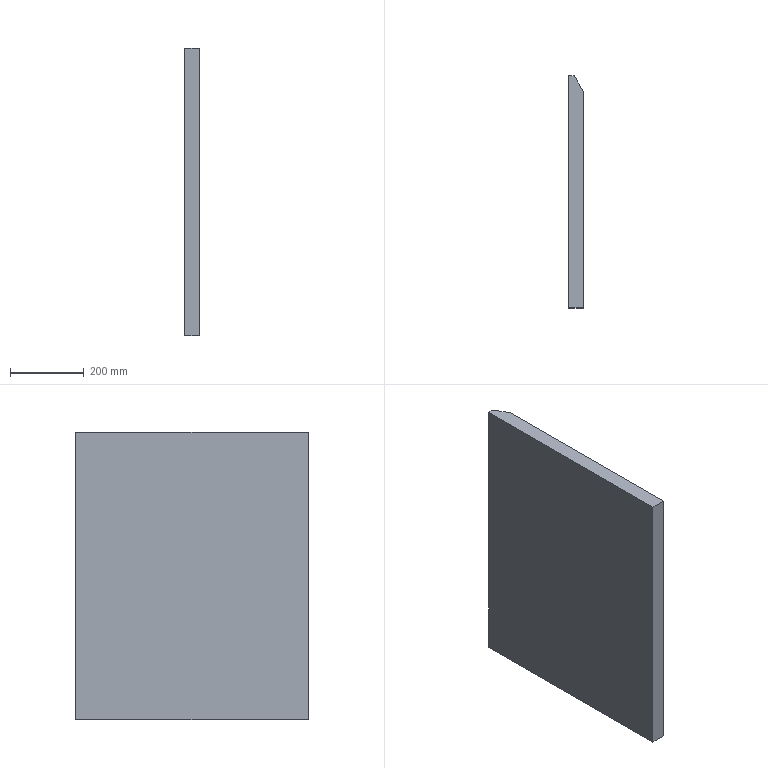Part | SolidWorks | features CutThin 1, Extrusion 1 | 1 solid | 17 faces | box 40 x 630 x 780 mm | volume 19233148 mm3 | plane 17
STEP:
#1=CARTESIAN_POINT('',(15.,0.,0.));
#2=VERTEX_POINT('',#1);
#3=CARTESIAN_POINT('',(0.,0.,0.));
#4=VERTEX_POINT('',#3);
#5=CARTESIAN_POINT('',(0.,0.,0.));
#6=DIRECTION('',(-1.,0.,0.));
#7=VECTOR('',#6,1000.);
#8=LINE('',#5,#7);
#9=EDGE_CURVE('',#2,#4,#8,.T.);
#10=ORIENTED_EDGE('',*,*,#9,.T.);
#11=CARTESIAN_POINT('',(0.,0.,780.));
#12=VERTEX_POINT('',#11);
#13=CARTESIAN_POINT('',(0.,0.,780.));
#14=DIRECTION('',(0.,0.,-1.));
#15=VECTOR('',#14,1000.);
#16=LINE('',#13,#15);
#17=EDGE_CURVE('',#12,#4,#16,.T.);
#18=ORIENTED_EDGE('',*,*,#17,.F.);
#19=CARTESIAN_POINT('',(15.,0.,780.));
#20=VERTEX_POINT('',#19);
#21=CARTESIAN_POINT('',(0.,0.,780.));
#22=DIRECTION('',(-1.,0.,0.));
#23=VECTOR('',#22,1000.);
#24=LINE('',#21,#23);
#25=EDGE_CURVE('',#20,#12,#24,.T.);
#26=ORIENTED_EDGE('',*,*,#25,.F.);
#27=CARTESIAN_POINT('',(15.,0.,780.));
#28=DIRECTION('',(0.,0.,-1.));
#29=VECTOR('',#28,1000.);
#30=LINE('',#27,#29);
#31=EDGE_CURVE('',#20,#2,#30,.T.);
#32=ORIENTED_EDGE('',*,*,#31,.T.);
#33=EDGE_LOOP('',(#10,#18,#26,#32));
#34=FACE_OUTER_BOUND('',#33,.T.);
#35=CARTESIAN_POINT('',(0.,0.,780.));
#36=DIRECTION('',(0.,-1.,0.));
#37=DIRECTION('',(0.,0.,-1.));
#38=AXIS2_PLACEMENT_3D('',#35,#36,#37);
#39=PLANE('',#38);
#40=ADVANCED_FACE('',(#34),#39,.F.);
#41=CARTESIAN_POINT('',(0.,-630.,0.));
#42=VERTEX_POINT('',#41);
#43=CARTESIAN_POINT('',(0.,0.,0.));
#44=DIRECTION('',(0.,-1.,0.));
#45=VECTOR('',#44,1000.);
#46=LINE('',#43,#45);
#47=EDGE_CURVE('',#4,#42,#46,.T.);
#48=ORIENTED_EDGE('',*,*,#47,.T.);
#49=CARTESIAN_POINT('',(0.,-630.,780.));
#50=VERTEX_POINT('',#49);
#51=CARTESIAN_POINT('',(0.,-630.,780.));
#52=DIRECTION('',(0.,0.,-1.));
#53=VECTOR('',#52,1000.);
#54=LINE('',#51,#53);
#55=EDGE_CURVE('',#50,#42,#54,.T.);
#56=ORIENTED_EDGE('',*,*,#55,.F.);
#57=CARTESIAN_POINT('',(0.,0.,780.));
#58=DIRECTION('',(0.,-1.,0.));
#59=VECTOR('',#58,1000.);
#60=LINE('',#57,#59);
#61=EDGE_CURVE('',#12,#50,#60,.T.);
#62=ORIENTED_EDGE('',*,*,#61,.F.);
#63=ORIENTED_EDGE('',*,*,#17,.T.);
#64=EDGE_LOOP('',(#48,#56,#62,#63));
#65=FACE_OUTER_BOUND('',#64,.T.);
#66=CARTESIAN_POINT('',(0.,0.,780.));
#67=DIRECTION('',(1.,0.,0.));
#68=DIRECTION('',(0.,1.,0.));
#69=AXIS2_PLACEMENT_3D('',#66,#67,#68);
#70=PLANE('',#69);
#71=ADVANCED_FACE('',(#65),#70,.F.);
#72=CARTESIAN_POINT('',(40.,-630.,0.));
#73=VERTEX_POINT('',#72);
#74=CARTESIAN_POINT('',(0.,-630.,0.));
#75=DIRECTION('',(1.,0.,0.));
#76=VECTOR('',#75,1000.);
#77=LINE('',#74,#76);
#78=EDGE_CURVE('',#42,#73,#77,.T.);
#79=ORIENTED_EDGE('',*,*,#78,.T.);
#80=CARTESIAN_POINT('',(40.,-630.,780.));
#81=VERTEX_POINT('',#80);
#82=CARTESIAN_POINT('',(40.,-630.,780.));
#83=DIRECTION('',(0.,0.,-1.));
#84=VECTOR('',#83,1000.);
#85=LINE('',#82,#84);
#86=EDGE_CURVE('',#81,#73,#85,.T.);
#87=ORIENTED_EDGE('',*,*,#86,.F.);
#88=CARTESIAN_POINT('',(0.,-630.,780.));
#89=DIRECTION('',(1.,0.,0.));
#90=VECTOR('',#89,1000.);
#91=LINE('',#88,#90);
#92=EDGE_CURVE('',#50,#81,#91,.T.);
#93=ORIENTED_EDGE('',*,*,#92,.F.);
#94=ORIENTED_EDGE('',*,*,#55,.T.);
#95=EDGE_LOOP('',(#79,#87,#93,#94));
#96=FACE_OUTER_BOUND('',#95,.T.);
#97=CARTESIAN_POINT('',(0.,-630.,780.));
#98=DIRECTION('',(0.,1.,0.));
#99=DIRECTION('',(0.,0.,1.));
#100=AXIS2_PLACEMENT_3D('',#97,#98,#99);
#101=PLANE('',#100);
#102=ADVANCED_FACE('',(#96),#101,.F.);
#103=CARTESIAN_POINT('',(40.,-144.501,439.2));
#104=VERTEX_POINT('',#103);
#105=CARTESIAN_POINT('',(40.,-144.501,340.8));
#106=VERTEX_POINT('',#105);
#107=CARTESIAN_POINT('',(40.,-144.501,438.));
#108=DIRECTION('',(0.,0.,-1.));
#109=VECTOR('',#108,1000.);
#110=LINE('',#107,#109);
#111=EDGE_CURVE('',#104,#106,#110,.T.);
#112=ORIENTED_EDGE('',*,*,#111,.F.);
#113=CARTESIAN_POINT('',(40.,-102.101,439.2));
#114=VERTEX_POINT('',#113);
#115=CARTESIAN_POINT('',(40.,-103.301,439.2));
#116=DIRECTION('',(0.,-1.,0.));
#117=VECTOR('',#116,1000.);
#118=LINE('',#115,#117);
#119=EDGE_CURVE('',#114,#104,#118,.T.);
#120=ORIENTED_EDGE('',*,*,#119,.F.);
#121=CARTESIAN_POINT('',(40.,-102.101,340.8));
#122=VERTEX_POINT('',#121);
#123=CARTESIAN_POINT('',(40.,-102.101,438.));
#124=DIRECTION('',(0.,0.,1.));
#125=VECTOR('',#124,1000.);
#126=LINE('',#123,#125);
#127=EDGE_CURVE('',#122,#114,#126,.T.);
#128=ORIENTED_EDGE('',*,*,#127,.F.);
#129=CARTESIAN_POINT('',(40.,-103.301,340.8));
#130=DIRECTION('',(0.,1.,0.));
#131=VECTOR('',#130,1000.);
#132=LINE('',#129,#131);
#133=EDGE_CURVE('',#106,#122,#132,.T.);
#134=ORIENTED_EDGE('',*,*,#133,.F.);
#135=EDGE_LOOP('',(#112,#120,#128,#134));
#136=FACE_BOUND('',#135,.T.);
#137=CARTESIAN_POINT('',(40.,-43.301,0.));
#138=VERTEX_POINT('',#137);
#139=CARTESIAN_POINT('',(40.,-630.,0.));
#140=DIRECTION('',(0.,1.,0.));
#141=VECTOR('',#140,1000.);
#142=LINE('',#139,#141);
#143=EDGE_CURVE('',#73,#138,#142,.T.);
#144=ORIENTED_EDGE('',*,*,#143,.T.);
#145=CARTESIAN_POINT('',(40.,-43.301,780.));
#146=VERTEX_POINT('',#145);
#147=CARTESIAN_POINT('',(40.,-43.301,780.));
#148=DIRECTION('',(0.,0.,-1.));
#149=VECTOR('',#148,1000.);
#150=LINE('',#147,#149);
#151=EDGE_CURVE('',#146,#138,#150,.T.);
#152=ORIENTED_EDGE('',*,*,#151,.F.);
#153=CARTESIAN_POINT('',(40.,-630.,780.));
#154=DIRECTION('',(0.,1.,0.));
#155=VECTOR('',#154,1000.);
#156=LINE('',#153,#155);
#157=EDGE_CURVE('',#81,#146,#156,.T.);
#158=ORIENTED_EDGE('',*,*,#157,.F.);
#159=ORIENTED_EDGE('',*,*,#86,.T.);
#160=EDGE_LOOP('',(#144,#152,#158,#159));
#161=FACE_OUTER_BOUND('',#160,.T.);
#162=CARTESIAN_POINT('',(40.,-630.,780.));
#163=DIRECTION('',(-1.,0.,0.));
#164=DIRECTION('',(0.,-1.,0.));
#165=AXIS2_PLACEMENT_3D('',#162,#163,#164);
#166=PLANE('',#165);
#167=ADVANCED_FACE('',(#136,#161),#166,.F.);
#168=CARTESIAN_POINT('',(15.,0.,0.));
#169=DIRECTION('',(-0.5,0.866,0.));
#170=VECTOR('',#169,1000.);
#171=LINE('',#168,#170);
#172=EDGE_CURVE('',#138,#2,#171,.T.);
#173=ORIENTED_EDGE('',*,*,#172,.T.);
#174=ORIENTED_EDGE('',*,*,#31,.F.);
#175=CARTESIAN_POINT('',(15.,0.,780.));
#176=DIRECTION('',(-0.5,0.866,0.));
#177=VECTOR('',#176,1000.);
#178=LINE('',#175,#177);
#179=EDGE_CURVE('',#146,#20,#178,.T.);
#180=ORIENTED_EDGE('',*,*,#179,.F.);
#181=ORIENTED_EDGE('',*,*,#151,.T.);
#182=EDGE_LOOP('',(#173,#174,#180,#181));
#183=FACE_OUTER_BOUND('',#182,.T.);
#184=CARTESIAN_POINT('',(15.,0.,780.));
#185=DIRECTION('',(-0.866,-0.5,0.));
#186=DIRECTION('',(0.5,-0.866,0.));
#187=AXIS2_PLACEMENT_3D('',#184,#185,#186);
#188=PLANE('',#187);
#189=ADVANCED_FACE('',(#183),#188,.F.);
#190=ORIENTED_EDGE('',*,*,#25,.T.);
#191=ORIENTED_EDGE('',*,*,#61,.T.);
#192=ORIENTED_EDGE('',*,*,#92,.T.);
#193=ORIENTED_EDGE('',*,*,#157,.T.);
#194=ORIENTED_EDGE('',*,*,#179,.T.);
#195=EDGE_LOOP('',(#190,#191,#192,#193,#194));
#196=FACE_OUTER_BOUND('',#195,.T.);
#197=CARTESIAN_POINT('',(0.,0.,780.));
#198=DIRECTION('',(0.,0.,1.));
#199=DIRECTION('',(1.,0.,0.));
#200=AXIS2_PLACEMENT_3D('',#197,#198,#199);
#201=PLANE('',#200);
#202=ADVANCED_FACE('',(#196),#201,.T.);
#203=ORIENTED_EDGE('',*,*,#9,.F.);
#204=ORIENTED_EDGE('',*,*,#172,.F.);
#205=ORIENTED_EDGE('',*,*,#143,.F.);
#206=ORIENTED_EDGE('',*,*,#78,.F.);
#207=ORIENTED_EDGE('',*,*,#47,.F.);
#208=EDGE_LOOP('',(#203,#204,#205,#206,#207));
#209=FACE_OUTER_BOUND('',#208,.T.);
#210=CARTESIAN_POINT('',(0.,0.,0.));
#211=DIRECTION('',(0.,0.,1.));
#212=DIRECTION('',(1.,0.,0.));
#213=AXIS2_PLACEMENT_3D('',#210,#211,#212);
#214=PLANE('',#213);
#215=ADVANCED_FACE('',(#209),#214,.F.);
#216=ORIENTED_EDGE('',*,*,#119,.T.);
#217=CARTESIAN_POINT('',(38.,-144.501,439.2));
#218=VERTEX_POINT('',#217);
#219=CARTESIAN_POINT('',(38.,-144.501,439.2));
#220=DIRECTION('',(1.,0.,0.));
#221=VECTOR('',#220,1000.);
#222=LINE('',#219,#221);
#223=EDGE_CURVE('',#218,#104,#222,.T.);
#224=ORIENTED_EDGE('',*,*,#223,.F.);
#225=CARTESIAN_POINT('',(38.,-102.101,439.2));
#226=VERTEX_POINT('',#225);
#227=CARTESIAN_POINT('',(38.,-103.301,439.2));
#228=DIRECTION('',(0.,-1.,0.));
#229=VECTOR('',#228,1000.);
#230=LINE('',#227,#229);
#231=EDGE_CURVE('',#226,#218,#230,.T.);
#232=ORIENTED_EDGE('',*,*,#231,.F.);
#233=CARTESIAN_POINT('',(38.,-102.101,439.2));
#234=DIRECTION('',(1.,0.,0.));
#235=VECTOR('',#234,1000.);
#236=LINE('',#233,#235);
#237=EDGE_CURVE('',#226,#114,#236,.T.);
#238=ORIENTED_EDGE('',*,*,#237,.T.);
#239=EDGE_LOOP('',(#216,#224,#232,#238));
#240=FACE_OUTER_BOUND('',#239,.T.);
#241=CARTESIAN_POINT('',(38.,-103.301,439.2));
#242=DIRECTION('',(0.,0.,1.));
#243=DIRECTION('',(1.,0.,0.));
#244=AXIS2_PLACEMENT_3D('',#241,#242,#243);
#245=PLANE('',#244);
#246=ADVANCED_FACE('',(#240),#245,.F.);
#247=ORIENTED_EDGE('',*,*,#127,.T.);
#248=ORIENTED_EDGE('',*,*,#237,.F.);
#249=CARTESIAN_POINT('',(38.,-102.101,340.8));
#250=VERTEX_POINT('',#249);
#251=CARTESIAN_POINT('',(38.,-102.101,438.));
#252=DIRECTION('',(0.,0.,1.));
#253=VECTOR('',#252,1000.);
#254=LINE('',#251,#253);
#255=EDGE_CURVE('',#250,#226,#254,.T.);
#256=ORIENTED_EDGE('',*,*,#255,.F.);
#257=CARTESIAN_POINT('',(38.,-102.101,340.8));
#258=DIRECTION('',(1.,0.,0.));
#259=VECTOR('',#258,1000.);
#260=LINE('',#257,#259);
#261=EDGE_CURVE('',#250,#122,#260,.T.);
#262=ORIENTED_EDGE('',*,*,#261,.T.);
#263=EDGE_LOOP('',(#247,#248,#256,#262));
#264=FACE_OUTER_BOUND('',#263,.T.);
#265=CARTESIAN_POINT('',(38.,-102.101,438.));
#266=DIRECTION('',(0.,1.,0.));
#267=DIRECTION('',(0.,0.,1.));
#268=AXIS2_PLACEMENT_3D('',#265,#266,#267);
#269=PLANE('',#268);
#270=ADVANCED_FACE('',(#264),#269,.F.);
#271=ORIENTED_EDGE('',*,*,#133,.T.);
#272=ORIENTED_EDGE('',*,*,#261,.F.);
#273=CARTESIAN_POINT('',(38.,-144.501,340.8));
#274=VERTEX_POINT('',#273);
#275=CARTESIAN_POINT('',(38.,-103.301,340.8));
#276=DIRECTION('',(0.,1.,0.));
#277=VECTOR('',#276,1000.);
#278=LINE('',#275,#277);
#279=EDGE_CURVE('',#274,#250,#278,.T.);
#280=ORIENTED_EDGE('',*,*,#279,.F.);
#281=CARTESIAN_POINT('',(38.,-144.501,340.8));
#282=DIRECTION('',(1.,0.,0.));
#283=VECTOR('',#282,1000.);
#284=LINE('',#281,#283);
#285=EDGE_CURVE('',#274,#106,#284,.T.);
#286=ORIENTED_EDGE('',*,*,#285,.T.);
#287=EDGE_LOOP('',(#271,#272,#280,#286));
#288=FACE_OUTER_BOUND('',#287,.T.);
#289=CARTESIAN_POINT('',(38.,-103.301,340.8));
#290=DIRECTION('',(0.,0.,-1.));
#291=DIRECTION('',(0.,1.,0.));
#292=AXIS2_PLACEMENT_3D('',#289,#290,#291);
#293=PLANE('',#292);
#294=ADVANCED_FACE('',(#288),#293,.F.);
#295=ORIENTED_EDGE('',*,*,#111,.T.);
#296=ORIENTED_EDGE('',*,*,#285,.F.);
#297=CARTESIAN_POINT('',(38.,-144.501,438.));
#298=DIRECTION('',(0.,0.,-1.));
#299=VECTOR('',#298,1000.);
#300=LINE('',#297,#299);
#301=EDGE_CURVE('',#218,#274,#300,.T.);
#302=ORIENTED_EDGE('',*,*,#301,.F.);
#303=ORIENTED_EDGE('',*,*,#223,.T.);
#304=EDGE_LOOP('',(#295,#296,#302,#303));
#305=FACE_OUTER_BOUND('',#304,.T.);
#306=CARTESIAN_POINT('',(38.,-144.501,438.));
#307=DIRECTION('',(0.,-1.,0.));
#308=DIRECTION('',(1.,0.,0.));
#309=AXIS2_PLACEMENT_3D('',#306,#307,#308);
#310=PLANE('',#309);
#311=ADVANCED_FACE('',(#305),#310,.F.);
#312=CARTESIAN_POINT('',(38.,-103.301,342.));
#313=VERTEX_POINT('',#312);
#314=CARTESIAN_POINT('',(38.,-103.301,438.));
#315=VERTEX_POINT('',#314);
#316=CARTESIAN_POINT('',(38.,-103.301,438.));
#317=DIRECTION('',(0.,0.,1.));
#318=VECTOR('',#317,1000.);
#319=LINE('',#316,#318);
#320=EDGE_CURVE('',#313,#315,#319,.T.);
#321=ORIENTED_EDGE('',*,*,#320,.F.);
#322=CARTESIAN_POINT('',(38.,-143.301,342.));
#323=VERTEX_POINT('',#322);
#324=CARTESIAN_POINT('',(38.,-103.301,342.));
#325=DIRECTION('',(0.,1.,0.));
#326=VECTOR('',#325,1000.);
#327=LINE('',#324,#326);
#328=EDGE_CURVE('',#323,#313,#327,.T.);
#329=ORIENTED_EDGE('',*,*,#328,.F.);
#330=CARTESIAN_POINT('',(38.,-143.301,438.));
#331=VERTEX_POINT('',#330);
#332=CARTESIAN_POINT('',(38.,-143.301,438.));
#333=DIRECTION('',(0.,0.,-1.));
#334=VECTOR('',#333,1000.);
#335=LINE('',#332,#334);
#336=EDGE_CURVE('',#331,#323,#335,.T.);
#337=ORIENTED_EDGE('',*,*,#336,.F.);
#338=CARTESIAN_POINT('',(38.,-103.301,438.));
#339=DIRECTION('',(0.,-1.,0.));
#340=VECTOR('',#339,1000.);
#341=LINE('',#338,#340);
#342=EDGE_CURVE('',#315,#331,#341,.T.);
#343=ORIENTED_EDGE('',*,*,#342,.F.);
#344=EDGE_LOOP('',(#321,#329,#337,#343));
#345=FACE_BOUND('',#344,.T.);
#346=ORIENTED_EDGE('',*,*,#231,.T.);
#347=ORIENTED_EDGE('',*,*,#301,.T.);
#348=ORIENTED_EDGE('',*,*,#279,.T.);
#349=ORIENTED_EDGE('',*,*,#255,.T.);
#350=EDGE_LOOP('',(#346,#347,#348,#349));
#351=FACE_OUTER_BOUND('',#350,.T.);
#352=CARTESIAN_POINT('',(38.,0.,0.));
#353=DIRECTION('',(1.,0.,0.));
#354=DIRECTION('',(0.,0.,-1.));
#355=AXIS2_PLACEMENT_3D('',#352,#353,#354);
#356=PLANE('',#355);
#357=ADVANCED_FACE('',(#345,#351),#356,.T.);
#358=CARTESIAN_POINT('',(40.,-103.301,438.));
#359=VERTEX_POINT('',#358);
#360=CARTESIAN_POINT('',(40.,-143.301,438.));
#361=VERTEX_POINT('',#360);
#362=CARTESIAN_POINT('',(40.,-103.301,438.));
#363=DIRECTION('',(0.,-1.,0.));
#364=VECTOR('',#363,1000.);
#365=LINE('',#362,#364);
#366=EDGE_CURVE('',#359,#361,#365,.T.);
#367=ORIENTED_EDGE('',*,*,#366,.F.);
#368=CARTESIAN_POINT('',(38.,-103.301,438.));
#369=DIRECTION('',(1.,0.,0.));
#370=VECTOR('',#369,1000.);
#371=LINE('',#368,#370);
#372=EDGE_CURVE('',#315,#359,#371,.T.);
#373=ORIENTED_EDGE('',*,*,#372,.F.);
#374=ORIENTED_EDGE('',*,*,#342,.T.);
#375=CARTESIAN_POINT('',(38.,-143.301,438.));
#376=DIRECTION('',(1.,0.,0.));
#377=VECTOR('',#376,1000.);
#378=LINE('',#375,#377);
#379=EDGE_CURVE('',#331,#361,#378,.T.);
#380=ORIENTED_EDGE('',*,*,#379,.T.);
#381=EDGE_LOOP('',(#367,#373,#374,#380));
#382=FACE_OUTER_BOUND('',#381,.T.);
#383=CARTESIAN_POINT('',(38.,-103.301,438.));
#384=DIRECTION('',(0.,0.,1.));
#385=DIRECTION('',(1.,0.,0.));
#386=AXIS2_PLACEMENT_3D('',#383,#384,#385);
#387=PLANE('',#386);
#388=ADVANCED_FACE('',(#382),#387,.T.);
#389=CARTESIAN_POINT('',(40.,-103.301,342.));
#390=VERTEX_POINT('',#389);
#391=CARTESIAN_POINT('',(40.,-103.301,438.));
#392=DIRECTION('',(0.,0.,1.));
#393=VECTOR('',#392,1000.);
#394=LINE('',#391,#393);
#395=EDGE_CURVE('',#390,#359,#394,.T.);
#396=ORIENTED_EDGE('',*,*,#395,.F.);
#397=CARTESIAN_POINT('',(38.,-103.301,342.));
#398=DIRECTION('',(1.,0.,0.));
#399=VECTOR('',#398,1000.);
#400=LINE('',#397,#399);
#401=EDGE_CURVE('',#313,#390,#400,.T.);
#402=ORIENTED_EDGE('',*,*,#401,.F.);
#403=ORIENTED_EDGE('',*,*,#320,.T.);
#404=ORIENTED_EDGE('',*,*,#372,.T.);
#405=EDGE_LOOP('',(#396,#402,#403,#404));
#406=FACE_OUTER_BOUND('',#405,.T.);
#407=CARTESIAN_POINT('',(38.,-103.301,438.));
#408=DIRECTION('',(0.,1.,0.));
#409=DIRECTION('',(0.,0.,1.));
#410=AXIS2_PLACEMENT_3D('',#407,#408,#409);
#411=PLANE('',#410);
#412=ADVANCED_FACE('',(#406),#411,.T.);
#413=CARTESIAN_POINT('',(40.,-143.301,342.));
#414=VERTEX_POINT('',#413);
#415=CARTESIAN_POINT('',(40.,-103.301,342.));
#416=DIRECTION('',(0.,1.,0.));
#417=VECTOR('',#416,1000.);
#418=LINE('',#415,#417);
#419=EDGE_CURVE('',#414,#390,#418,.T.);
#420=ORIENTED_EDGE('',*,*,#419,.F.);
#421=CARTESIAN_POINT('',(38.,-143.301,342.));
#422=DIRECTION('',(1.,0.,0.));
#423=VECTOR('',#422,1000.);
#424=LINE('',#421,#423);
#425=EDGE_CURVE('',#323,#414,#424,.T.);
#426=ORIENTED_EDGE('',*,*,#425,.F.);
#427=ORIENTED_EDGE('',*,*,#328,.T.);
#428=ORIENTED_EDGE('',*,*,#401,.T.);
#429=EDGE_LOOP('',(#420,#426,#427,#428));
#430=FACE_OUTER_BOUND('',#429,.T.);
#431=CARTESIAN_POINT('',(38.,-103.301,342.));
#432=DIRECTION('',(0.,0.,-1.));
#433=DIRECTION('',(0.,1.,0.));
#434=AXIS2_PLACEMENT_3D('',#431,#432,#433);
#435=PLANE('',#434);
#436=ADVANCED_FACE('',(#430),#435,.T.);
#437=CARTESIAN_POINT('',(40.,-143.301,438.));
#438=DIRECTION('',(0.,0.,-1.));
#439=VECTOR('',#438,1000.);
#440=LINE('',#437,#439);
#441=EDGE_CURVE('',#361,#414,#440,.T.);
#442=ORIENTED_EDGE('',*,*,#441,.F.);
#443=ORIENTED_EDGE('',*,*,#379,.F.);
#444=ORIENTED_EDGE('',*,*,#336,.T.);
#445=ORIENTED_EDGE('',*,*,#425,.T.);
#446=EDGE_LOOP('',(#442,#443,#444,#445));
#447=FACE_OUTER_BOUND('',#446,.T.);
#448=CARTESIAN_POINT('',(38.,-143.301,438.));
#449=DIRECTION('',(0.,-1.,0.));
#450=DIRECTION('',(1.,0.,0.));
#451=AXIS2_PLACEMENT_3D('',#448,#449,#450);
#452=PLANE('',#451);
#453=ADVANCED_FACE('',(#447),#452,.T.);
#454=ORIENTED_EDGE('',*,*,#366,.T.);
#455=ORIENTED_EDGE('',*,*,#441,.T.);
#456=ORIENTED_EDGE('',*,*,#419,.T.);
#457=ORIENTED_EDGE('',*,*,#395,.T.);
#458=EDGE_LOOP('',(#454,#455,#456,#457));
#459=FACE_OUTER_BOUND('',#458,.T.);
#460=CARTESIAN_POINT('',(40.,-630.,780.));
#461=DIRECTION('',(-1.,0.,0.));
#462=DIRECTION('',(0.,-1.,0.));
#463=AXIS2_PLACEMENT_3D('',#460,#461,#462);
#464=PLANE('',#463);
#465=ADVANCED_FACE('',(#459),#464,.F.);
#466=CLOSED_SHELL('',(#40,#71,#102,#167,#189,#202,#215,#246,#270,#294,#311,#357,#388,#412,#436,#453,#465));
#467=MANIFOLD_SOLID_BREP('',#466);
#468=CARTESIAN_POINT('',(0.,0.,0.));
#469=DIRECTION('',(0.,0.,1.));
#470=DIRECTION('',(1.,0.,0.));
#471=AXIS2_PLACEMENT_3D('',#468,#469,#470);
#472=(LENGTH_UNIT()NAMED_UNIT(*)SI_UNIT(.MILLI.,.METRE.));
#473=UNCERTAINTY_MEASURE_WITH_UNIT(LENGTH_MEASURE(0.00001),#472,'','');
#474=(NAMED_UNIT(*)PLANE_ANGLE_UNIT()SI_UNIT($,.RADIAN.));
#475=(NAMED_UNIT(*)SI_UNIT($,.STERADIAN.)SOLID_ANGLE_UNIT());
#476=(GEOMETRIC_REPRESENTATION_CONTEXT(3)GLOBAL_UNCERTAINTY_ASSIGNED_CONTEXT((#473))GLOBAL_UNIT_ASSIGNED_CONTEXT((#472,#474,#475))REPRESENTATION_CONTEXT('',''));
#477=ADVANCED_BREP_SHAPE_REPRESENTATION('',(#467,#471),#476);